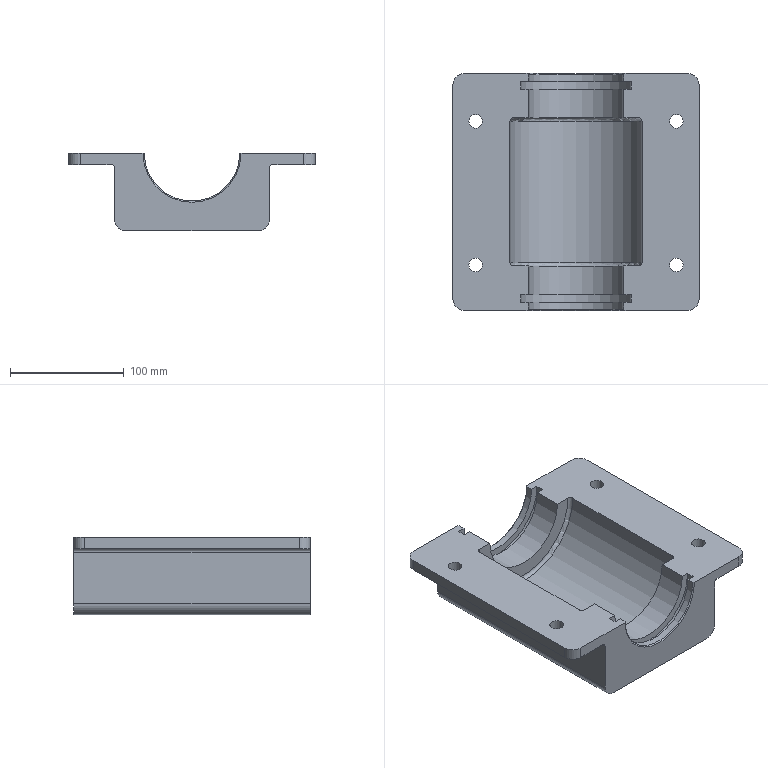Part | NX | features DATUM_CSYS 10, SKETCH 9, EXTRACT_FACE 6, HOLE PACKAGE 6, SIMPLE HOLE 6, BLEND 4, Instance Feature 4, EXTRUDE 2, Pattern Feature 2, SYMBOLIC_THREAD 2, CHAMFER 1, DATUM_PLANE 1, SWP104 1 | 1 solid | 44 faces | box 216 x 208 x 68 mm | volume 1158668 mm3 | cylinder 21 | plane 17 | cone 4 | torus 2 | commonest cylinder face diameters 20 x6 12 x4 84 x4 6 x2 8.5 x2 97 x2
STEP:
#1=CARTESIAN_POINT('',(166.,0.,68.));
#2=VERTEX_POINT('',#1);
#3=CARTESIAN_POINT('',(111.,0.,68.));
#4=VERTEX_POINT('',#3);
#5=CARTESIAN_POINT('',(176.,0.,68.));
#6=DIRECTION('',(-1.,0.,0.));
#7=VECTOR('',#6,1000.);
#8=LINE('',#5,#7);
#9=EDGE_CURVE('',#2,#4,#8,.T.);
#10=ORIENTED_EDGE('',*,*,#9,.T.);
#11=CARTESIAN_POINT('',(25.,0.,68.));
#12=VERTEX_POINT('',#11);
#13=CARTESIAN_POINT('',(68.,0.,68.));
#14=DIRECTION('',(0.,1.,0.));
#15=DIRECTION('',(-1.,0.,0.));
#16=AXIS2_PLACEMENT_3D('',#13,#14,#15);
#17=CIRCLE('',#16,43.);
#18=EDGE_CURVE('',#4,#12,#17,.T.);
#19=ORIENTED_EDGE('',*,*,#18,.T.);
#20=CARTESIAN_POINT('',(-30.,0.,68.));
#21=VERTEX_POINT('',#20);
#22=CARTESIAN_POINT('',(176.,0.,68.));
#23=DIRECTION('',(-1.,0.,0.));
#24=VECTOR('',#23,1000.);
#25=LINE('',#22,#24);
#26=EDGE_CURVE('',#12,#21,#25,.T.);
#27=ORIENTED_EDGE('',*,*,#26,.T.);
#28=CARTESIAN_POINT('',(-30.,0.,58.));
#29=VERTEX_POINT('',#28);
#30=CARTESIAN_POINT('',(-30.,0.,58.));
#31=DIRECTION('',(0.,0.,-1.));
#32=VECTOR('',#31,1000.);
#33=LINE('',#30,#32);
#34=EDGE_CURVE('',#21,#29,#33,.T.);
#35=ORIENTED_EDGE('',*,*,#34,.T.);
#36=CARTESIAN_POINT('',(-3.,0.,58.));
#37=VERTEX_POINT('',#36);
#38=CARTESIAN_POINT('',(-40.,0.,58.));
#39=DIRECTION('',(1.,0.,0.));
#40=VECTOR('',#39,1000.);
#41=LINE('',#38,#40);
#42=EDGE_CURVE('',#29,#37,#41,.T.);
#43=ORIENTED_EDGE('',*,*,#42,.T.);
#44=CARTESIAN_POINT('',(0.,0.,55.));
#45=VERTEX_POINT('',#44);
#46=CARTESIAN_POINT('',(-3.,0.,55.));
#47=DIRECTION('',(0.,1.,0.));
#48=DIRECTION('',(-1.,0.,0.));
#49=AXIS2_PLACEMENT_3D('',#46,#47,#48);
#50=CIRCLE('',#49,3.);
#51=EDGE_CURVE('',#37,#45,#50,.T.);
#52=ORIENTED_EDGE('',*,*,#51,.T.);
#53=CARTESIAN_POINT('',(0.,0.,10.));
#54=VERTEX_POINT('',#53);
#55=CARTESIAN_POINT('',(0.,0.,10.));
#56=DIRECTION('',(0.,0.,-1.));
#57=VECTOR('',#56,1000.);
#58=LINE('',#55,#57);
#59=EDGE_CURVE('',#45,#54,#58,.T.);
#60=ORIENTED_EDGE('',*,*,#59,.T.);
#61=CARTESIAN_POINT('',(10.,0.,0.));
#62=VERTEX_POINT('',#61);
#63=CARTESIAN_POINT('',(10.,0.,10.));
#64=DIRECTION('',(0.,1.,0.));
#65=DIRECTION('',(-1.,0.,0.));
#66=AXIS2_PLACEMENT_3D('',#63,#64,#65);
#67=CIRCLE('',#66,10.);
#68=EDGE_CURVE('',#54,#62,#67,.F.);
#69=ORIENTED_EDGE('',*,*,#68,.T.);
#70=CARTESIAN_POINT('',(126.,0.,0.));
#71=VERTEX_POINT('',#70);
#72=CARTESIAN_POINT('',(0.,0.,0.));
#73=DIRECTION('',(1.,0.,0.));
#74=VECTOR('',#73,1000.);
#75=LINE('',#72,#74);
#76=EDGE_CURVE('',#62,#71,#75,.T.);
#77=ORIENTED_EDGE('',*,*,#76,.T.);
#78=CARTESIAN_POINT('',(136.,0.,10.));
#79=VERTEX_POINT('',#78);
#80=CARTESIAN_POINT('',(126.,0.,10.));
#81=DIRECTION('',(0.,1.,0.));
#82=DIRECTION('',(-1.,0.,0.));
#83=AXIS2_PLACEMENT_3D('',#80,#81,#82);
#84=CIRCLE('',#83,10.);
#85=EDGE_CURVE('',#71,#79,#84,.F.);
#86=ORIENTED_EDGE('',*,*,#85,.T.);
#87=CARTESIAN_POINT('',(136.,0.,55.));
#88=VERTEX_POINT('',#87);
#89=CARTESIAN_POINT('',(136.,0.,10.));
#90=DIRECTION('',(0.,0.,-1.));
#91=VECTOR('',#90,1000.);
#92=LINE('',#89,#91);
#93=EDGE_CURVE('',#88,#79,#92,.T.);
#94=ORIENTED_EDGE('',*,*,#93,.F.);
#95=CARTESIAN_POINT('',(139.,0.,58.));
#96=VERTEX_POINT('',#95);
#97=CARTESIAN_POINT('',(139.,0.,55.));
#98=DIRECTION('',(0.,1.,0.));
#99=DIRECTION('',(-1.,0.,0.));
#100=AXIS2_PLACEMENT_3D('',#97,#98,#99);
#101=CIRCLE('',#100,3.);
#102=EDGE_CURVE('',#88,#96,#101,.T.);
#103=ORIENTED_EDGE('',*,*,#102,.T.);
#104=CARTESIAN_POINT('',(166.,0.,58.));
#105=VERTEX_POINT('',#104);
#106=CARTESIAN_POINT('',(136.,0.,58.));
#107=DIRECTION('',(1.,0.,0.));
#108=VECTOR('',#107,1000.);
#109=LINE('',#106,#108);
#110=EDGE_CURVE('',#96,#105,#109,.T.);
#111=ORIENTED_EDGE('',*,*,#110,.T.);
#112=CARTESIAN_POINT('',(166.,0.,68.));
#113=DIRECTION('',(0.,0.,1.));
#114=VECTOR('',#113,1000.);
#115=LINE('',#112,#114);
#116=EDGE_CURVE('',#105,#2,#115,.T.);
#117=ORIENTED_EDGE('',*,*,#116,.T.);
#118=EDGE_LOOP('',(#10,#19,#27,#35,#43,#52,#60,#69,#77,#86,#94,#103,#111,#117));
#119=FACE_BOUND('',#118,.T.);
#120=CARTESIAN_POINT('',(0.,0.,10.));
#121=DIRECTION('',(0.,1.,0.));
#122=DIRECTION('',(-1.,0.,0.));
#123=AXIS2_PLACEMENT_3D('',#120,#121,#122);
#124=PLANE('',#123);
#125=ADVANCED_FACE('',(#119),#124,.F.);
#126=CARTESIAN_POINT('',(-26.,166.,68.));
#127=VERTEX_POINT('',#126);
#128=CARTESIAN_POINT('',(-20.,166.,68.));
#129=DIRECTION('',(0.,0.,-1.));
#130=DIRECTION('',(-1.,0.,0.));
#131=AXIS2_PLACEMENT_3D('',#128,#129,#130);
#132=CIRCLE('',#131,6.);
#133=EDGE_CURVE('',#127,#127,#132,.T.);
#134=ORIENTED_EDGE('',*,*,#133,.T.);
#135=EDGE_LOOP('',(#134));
#136=FACE_BOUND('',#135,.T.);
#137=CARTESIAN_POINT('',(-26.,40.,68.));
#138=VERTEX_POINT('',#137);
#139=CARTESIAN_POINT('',(-20.,40.,68.));
#140=DIRECTION('',(0.,0.,-1.));
#141=DIRECTION('',(-1.,0.,0.));
#142=AXIS2_PLACEMENT_3D('',#139,#140,#141);
#143=CIRCLE('',#142,6.);
#144=EDGE_CURVE('',#138,#138,#143,.T.);
#145=ORIENTED_EDGE('',*,*,#144,.T.);
#146=EDGE_LOOP('',(#145));
#147=FACE_BOUND('',#146,.T.);
#148=ORIENTED_EDGE('',*,*,#26,.F.);
#149=CARTESIAN_POINT('',(26.,1.,68.));
#150=VERTEX_POINT('',#149);
#151=CARTESIAN_POINT('',(68.,43.,68.));
#152=DIRECTION('',(-0.7071,-0.7071,0.));
#153=VECTOR('',#152,1000.);
#154=LINE('',#151,#153);
#155=EDGE_CURVE('',#12,#150,#154,.F.);
#156=ORIENTED_EDGE('',*,*,#155,.T.);
#157=CARTESIAN_POINT('',(26.,7.,68.));
#158=VERTEX_POINT('',#157);
#159=CARTESIAN_POINT('',(26.,0.,68.));
#160=DIRECTION('',(0.,-1.,0.));
#161=VECTOR('',#160,1000.);
#162=LINE('',#159,#161);
#163=EDGE_CURVE('',#158,#150,#162,.T.);
#164=ORIENTED_EDGE('',*,*,#163,.F.);
#165=CARTESIAN_POINT('',(19.5,7.,68.));
#166=VERTEX_POINT('',#165);
#167=CARTESIAN_POINT('',(176.,7.,68.));
#168=DIRECTION('',(1.,0.,0.));
#169=VECTOR('',#168,1000.);
#170=LINE('',#167,#169);
#171=EDGE_CURVE('',#166,#158,#170,.T.);
#172=ORIENTED_EDGE('',*,*,#171,.F.);
#173=CARTESIAN_POINT('',(19.5,14.,68.));
#174=VERTEX_POINT('',#173);
#175=CARTESIAN_POINT('',(19.5,0.,68.));
#176=DIRECTION('',(0.,-1.,0.));
#177=VECTOR('',#176,1000.);
#178=LINE('',#175,#177);
#179=EDGE_CURVE('',#174,#166,#178,.T.);
#180=ORIENTED_EDGE('',*,*,#179,.F.);
#181=CARTESIAN_POINT('',(26.,14.,68.));
#182=VERTEX_POINT('',#181);
#183=CARTESIAN_POINT('',(176.,14.,68.));
#184=DIRECTION('',(-1.,0.,0.));
#185=VECTOR('',#184,1000.);
#186=LINE('',#183,#185);
#187=EDGE_CURVE('',#182,#174,#186,.T.);
#188=ORIENTED_EDGE('',*,*,#187,.F.);
#189=CARTESIAN_POINT('',(26.,39.,68.));
#190=VERTEX_POINT('',#189);
#191=CARTESIAN_POINT('',(26.,0.,68.));
#192=DIRECTION('',(0.,-1.,0.));
#193=VECTOR('',#192,1000.);
#194=LINE('',#191,#193);
#195=EDGE_CURVE('',#190,#182,#194,.T.);
#196=ORIENTED_EDGE('',*,*,#195,.F.);
#197=CARTESIAN_POINT('',(13.,39.,68.));
#198=VERTEX_POINT('',#197);
#199=CARTESIAN_POINT('',(176.,39.,68.));
#200=DIRECTION('',(1.,0.,0.));
#201=VECTOR('',#200,1000.);
#202=LINE('',#199,#201);
#203=EDGE_CURVE('',#198,#190,#202,.T.);
#204=ORIENTED_EDGE('',*,*,#203,.F.);
#205=CARTESIAN_POINT('',(10.,42.,68.));
#206=VERTEX_POINT('',#205);
#207=CARTESIAN_POINT('',(13.,42.,68.));
#208=DIRECTION('',(0.,0.,1.));
#209=DIRECTION('',(1.,0.,0.));
#210=AXIS2_PLACEMENT_3D('',#207,#208,#209);
#211=CIRCLE('',#210,3.);
#212=EDGE_CURVE('',#198,#206,#211,.F.);
#213=ORIENTED_EDGE('',*,*,#212,.T.);
#214=CARTESIAN_POINT('',(10.,166.,68.));
#215=VERTEX_POINT('',#214);
#216=CARTESIAN_POINT('',(10.,0.,68.));
#217=DIRECTION('',(0.,-1.,0.));
#218=VECTOR('',#217,1000.);
#219=LINE('',#216,#218);
#220=EDGE_CURVE('',#215,#206,#219,.T.);
#221=ORIENTED_EDGE('',*,*,#220,.F.);
#222=CARTESIAN_POINT('',(13.,169.,68.));
#223=VERTEX_POINT('',#222);
#224=CARTESIAN_POINT('',(13.,166.,68.));
#225=DIRECTION('',(0.,0.,1.));
#226=DIRECTION('',(1.,0.,0.));
#227=AXIS2_PLACEMENT_3D('',#224,#225,#226);
#228=CIRCLE('',#227,3.);
#229=EDGE_CURVE('',#215,#223,#228,.F.);
#230=ORIENTED_EDGE('',*,*,#229,.T.);
#231=CARTESIAN_POINT('',(26.,169.,68.));
#232=VERTEX_POINT('',#231);
#233=CARTESIAN_POINT('',(176.,169.,68.));
#234=DIRECTION('',(-1.,0.,0.));
#235=VECTOR('',#234,1000.);
#236=LINE('',#233,#235);
#237=EDGE_CURVE('',#232,#223,#236,.T.);
#238=ORIENTED_EDGE('',*,*,#237,.F.);
#239=CARTESIAN_POINT('',(26.,194.,68.));
#240=VERTEX_POINT('',#239);
#241=CARTESIAN_POINT('',(26.,0.,68.));
#242=DIRECTION('',(0.,-1.,0.));
#243=VECTOR('',#242,1000.);
#244=LINE('',#241,#243);
#245=EDGE_CURVE('',#240,#232,#244,.T.);
#246=ORIENTED_EDGE('',*,*,#245,.F.);
#247=CARTESIAN_POINT('',(19.5,194.,68.));
#248=VERTEX_POINT('',#247);
#249=CARTESIAN_POINT('',(176.,194.,68.));
#250=DIRECTION('',(1.,0.,0.));
#251=VECTOR('',#250,1000.);
#252=LINE('',#249,#251);
#253=EDGE_CURVE('',#248,#240,#252,.T.);
#254=ORIENTED_EDGE('',*,*,#253,.F.);
#255=CARTESIAN_POINT('',(19.5,201.,68.));
#256=VERTEX_POINT('',#255);
#257=CARTESIAN_POINT('',(19.5,0.,68.));
#258=DIRECTION('',(0.,-1.,0.));
#259=VECTOR('',#258,1000.);
#260=LINE('',#257,#259);
#261=EDGE_CURVE('',#256,#248,#260,.T.);
#262=ORIENTED_EDGE('',*,*,#261,.F.);
#263=CARTESIAN_POINT('',(26.,201.,68.));
#264=VERTEX_POINT('',#263);
#265=CARTESIAN_POINT('',(176.,201.,68.));
#266=DIRECTION('',(-1.,0.,0.));
#267=VECTOR('',#266,1000.);
#268=LINE('',#265,#267);
#269=EDGE_CURVE('',#264,#256,#268,.T.);
#270=ORIENTED_EDGE('',*,*,#269,.F.);
#271=CARTESIAN_POINT('',(26.,207.,68.));
#272=VERTEX_POINT('',#271);
#273=CARTESIAN_POINT('',(26.,0.,68.));
#274=DIRECTION('',(0.,-1.,0.));
#275=VECTOR('',#274,1000.);
#276=LINE('',#273,#275);
#277=EDGE_CURVE('',#272,#264,#276,.T.);
#278=ORIENTED_EDGE('',*,*,#277,.F.);
#279=CARTESIAN_POINT('',(25.,208.,68.));
#280=VERTEX_POINT('',#279);
#281=CARTESIAN_POINT('',(68.,165.,68.));
#282=DIRECTION('',(0.7071,-0.7071,0.));
#283=VECTOR('',#282,1000.);
#284=LINE('',#281,#283);
#285=EDGE_CURVE('',#272,#280,#284,.F.);
#286=ORIENTED_EDGE('',*,*,#285,.T.);
#287=CARTESIAN_POINT('',(-30.,208.,68.));
#288=VERTEX_POINT('',#287);
#289=CARTESIAN_POINT('',(176.,208.,68.));
#290=DIRECTION('',(-1.,0.,0.));
#291=VECTOR('',#290,1000.);
#292=LINE('',#289,#291);
#293=EDGE_CURVE('',#280,#288,#292,.T.);
#294=ORIENTED_EDGE('',*,*,#293,.T.);
#295=CARTESIAN_POINT('',(-40.,198.,68.));
#296=VERTEX_POINT('',#295);
#297=CARTESIAN_POINT('',(-30.,198.,68.));
#298=DIRECTION('',(0.,0.,1.));
#299=DIRECTION('',(1.,0.,0.));
#300=AXIS2_PLACEMENT_3D('',#297,#298,#299);
#301=CIRCLE('',#300,10.);
#302=EDGE_CURVE('',#288,#296,#301,.T.);
#303=ORIENTED_EDGE('',*,*,#302,.T.);
#304=CARTESIAN_POINT('',(-40.,10.,68.));
#305=VERTEX_POINT('',#304);
#306=CARTESIAN_POINT('',(-40.,208.,68.));
#307=DIRECTION('',(0.,-1.,0.));
#308=VECTOR('',#307,1000.);
#309=LINE('',#306,#308);
#310=EDGE_CURVE('',#296,#305,#309,.T.);
#311=ORIENTED_EDGE('',*,*,#310,.T.);
#312=CARTESIAN_POINT('',(-30.,10.,68.));
#313=DIRECTION('',(0.,0.,1.));
#314=DIRECTION('',(1.,0.,0.));
#315=AXIS2_PLACEMENT_3D('',#312,#313,#314);
#316=CIRCLE('',#315,10.);
#317=EDGE_CURVE('',#305,#21,#316,.T.);
#318=ORIENTED_EDGE('',*,*,#317,.T.);
#319=EDGE_LOOP('',(#148,#156,#164,#172,#180,#188,#196,#204,#213,#221,#230,#238,#246,#254,#262,#270,#278,#286,#294,#303,#311,#318));
#320=FACE_BOUND('',#319,.T.);
#321=CARTESIAN_POINT('',(176.,208.,68.));
#322=DIRECTION('',(0.,0.,1.));
#323=DIRECTION('',(1.,0.,0.));
#324=AXIS2_PLACEMENT_3D('',#321,#322,#323);
#325=PLANE('',#324);
#326=ADVANCED_FACE('',(#136,#147,#320),#325,.T.);
#327=ORIENTED_EDGE('',*,*,#59,.F.);
#328=CARTESIAN_POINT('',(0.,208.,55.));
#329=VERTEX_POINT('',#328);
#330=CARTESIAN_POINT('',(0.,208.,55.));
#331=DIRECTION('',(0.,-1.,0.));
#332=VECTOR('',#331,1000.);
#333=LINE('',#330,#332);
#334=EDGE_CURVE('',#45,#329,#333,.F.);
#335=ORIENTED_EDGE('',*,*,#334,.T.);
#336=CARTESIAN_POINT('',(0.,208.,10.));
#337=VERTEX_POINT('',#336);
#338=CARTESIAN_POINT('',(0.,208.,10.));
#339=DIRECTION('',(0.,0.,-1.));
#340=VECTOR('',#339,1000.);
#341=LINE('',#338,#340);
#342=EDGE_CURVE('',#329,#337,#341,.T.);
#343=ORIENTED_EDGE('',*,*,#342,.T.);
#344=CARTESIAN_POINT('',(0.,208.,10.));
#345=DIRECTION('',(0.,-1.,0.));
#346=VECTOR('',#345,1000.);
#347=LINE('',#344,#346);
#348=EDGE_CURVE('',#337,#54,#347,.T.);
#349=ORIENTED_EDGE('',*,*,#348,.T.);
#350=EDGE_LOOP('',(#327,#335,#343,#349));
#351=FACE_BOUND('',#350,.T.);
#352=CARTESIAN_POINT('',(0.,208.,10.));
#353=DIRECTION('',(1.,0.,0.));
#354=DIRECTION('',(0.,1.,0.));
#355=AXIS2_PLACEMENT_3D('',#352,#353,#354);
#356=PLANE('',#355);
#357=ADVANCED_FACE('',(#351),#356,.F.);
#358=CARTESIAN_POINT('',(136.,208.,55.));
#359=VERTEX_POINT('',#358);
#360=CARTESIAN_POINT('',(136.,208.,10.));
#361=VERTEX_POINT('',#360);
#362=CARTESIAN_POINT('',(136.,208.,10.));
#363=DIRECTION('',(0.,0.,-1.));
#364=VECTOR('',#363,1000.);
#365=LINE('',#362,#364);
#366=EDGE_CURVE('',#359,#361,#365,.T.);
#367=ORIENTED_EDGE('',*,*,#366,.F.);
#368=CARTESIAN_POINT('',(136.,0.,55.));
#369=DIRECTION('',(0.,-1.,0.));
#370=VECTOR('',#369,1000.);
#371=LINE('',#368,#370);
#372=EDGE_CURVE('',#359,#88,#371,.T.);
#373=ORIENTED_EDGE('',*,*,#372,.T.);
#374=ORIENTED_EDGE('',*,*,#93,.T.);
#375=CARTESIAN_POINT('',(136.,0.,10.));
#376=DIRECTION('',(0.,1.,0.));
#377=VECTOR('',#376,1000.);
#378=LINE('',#375,#377);
#379=EDGE_CURVE('',#79,#361,#378,.T.);
#380=ORIENTED_EDGE('',*,*,#379,.T.);
#381=EDGE_LOOP('',(#367,#373,#374,#380));
#382=FACE_BOUND('',#381,.T.);
#383=CARTESIAN_POINT('',(136.,0.,10.));
#384=DIRECTION('',(-1.,0.,0.));
#385=DIRECTION('',(0.,0.,1.));
#386=AXIS2_PLACEMENT_3D('',#383,#384,#385);
#387=PLANE('',#386);
#388=ADVANCED_FACE('',(#382),#387,.F.);
#389=ORIENTED_EDGE('',*,*,#293,.F.);
#390=CARTESIAN_POINT('',(111.,208.,68.));
#391=VERTEX_POINT('',#390);
#392=CARTESIAN_POINT('',(68.,208.,68.));
#393=DIRECTION('',(0.,-1.,0.));
#394=DIRECTION('',(1.,0.,0.));
#395=AXIS2_PLACEMENT_3D('',#392,#393,#394);
#396=CIRCLE('',#395,43.);
#397=EDGE_CURVE('',#280,#391,#396,.T.);
#398=ORIENTED_EDGE('',*,*,#397,.T.);
#399=CARTESIAN_POINT('',(166.,208.,68.));
#400=VERTEX_POINT('',#399);
#401=CARTESIAN_POINT('',(176.,208.,68.));
#402=DIRECTION('',(-1.,0.,0.));
#403=VECTOR('',#402,1000.);
#404=LINE('',#401,#403);
#405=EDGE_CURVE('',#400,#391,#404,.T.);
#406=ORIENTED_EDGE('',*,*,#405,.F.);
#407=CARTESIAN_POINT('',(166.,208.,58.));
#408=VERTEX_POINT('',#407);
#409=CARTESIAN_POINT('',(166.,208.,58.));
#410=DIRECTION('',(0.,0.,1.));
#411=VECTOR('',#410,1000.);
#412=LINE('',#409,#411);
#413=EDGE_CURVE('',#400,#408,#412,.F.);
#414=ORIENTED_EDGE('',*,*,#413,.T.);
#415=CARTESIAN_POINT('',(139.,208.,58.));
#416=VERTEX_POINT('',#415);
#417=CARTESIAN_POINT('',(136.,208.,58.));
#418=DIRECTION('',(1.,0.,0.));
#419=VECTOR('',#418,1000.);
#420=LINE('',#417,#419);
#421=EDGE_CURVE('',#416,#408,#420,.T.);
#422=ORIENTED_EDGE('',*,*,#421,.F.);
#423=CARTESIAN_POINT('',(139.,208.,55.));
#424=DIRECTION('',(0.,-1.,0.));
#425=DIRECTION('',(1.,0.,0.));
#426=AXIS2_PLACEMENT_3D('',#423,#424,#425);
#427=CIRCLE('',#426,3.);
#428=EDGE_CURVE('',#416,#359,#427,.T.);
#429=ORIENTED_EDGE('',*,*,#428,.T.);
#430=ORIENTED_EDGE('',*,*,#366,.T.);
#431=CARTESIAN_POINT('',(126.,208.,0.));
#432=VERTEX_POINT('',#431);
#433=CARTESIAN_POINT('',(126.,208.,10.));
#434=DIRECTION('',(0.,-1.,0.));
#435=DIRECTION('',(1.,0.,0.));
#436=AXIS2_PLACEMENT_3D('',#433,#434,#435);
#437=CIRCLE('',#436,10.);
#438=EDGE_CURVE('',#361,#432,#437,.F.);
#439=ORIENTED_EDGE('',*,*,#438,.T.);
#440=CARTESIAN_POINT('',(10.,208.,0.));
#441=VERTEX_POINT('',#440);
#442=CARTESIAN_POINT('',(136.,208.,0.));
#443=DIRECTION('',(-1.,0.,0.));
#444=VECTOR('',#443,1000.);
#445=LINE('',#442,#444);
#446=EDGE_CURVE('',#432,#441,#445,.T.);
#447=ORIENTED_EDGE('',*,*,#446,.T.);
#448=CARTESIAN_POINT('',(10.,208.,10.));
#449=DIRECTION('',(0.,-1.,0.));
#450=DIRECTION('',(1.,0.,0.));
#451=AXIS2_PLACEMENT_3D('',#448,#449,#450);
#452=CIRCLE('',#451,10.);
#453=EDGE_CURVE('',#441,#337,#452,.F.);
#454=ORIENTED_EDGE('',*,*,#453,.T.);
#455=ORIENTED_EDGE('',*,*,#342,.F.);
#456=CARTESIAN_POINT('',(-3.,208.,58.));
#457=VERTEX_POINT('',#456);
#458=CARTESIAN_POINT('',(-3.,208.,55.));
#459=DIRECTION('',(0.,-1.,0.));
#460=DIRECTION('',(1.,0.,0.));
#461=AXIS2_PLACEMENT_3D('',#458,#459,#460);
#462=CIRCLE('',#461,3.);
#463=EDGE_CURVE('',#329,#457,#462,.T.);
#464=ORIENTED_EDGE('',*,*,#463,.T.);
#465=CARTESIAN_POINT('',(-30.,208.,58.));
#466=VERTEX_POINT('',#465);
#467=CARTESIAN_POINT('',(-40.,208.,58.));
#468=DIRECTION('',(1.,0.,0.));
#469=VECTOR('',#468,1000.);
#470=LINE('',#467,#469);
#471=EDGE_CURVE('',#466,#457,#470,.T.);
#472=ORIENTED_EDGE('',*,*,#471,.F.);
#473=CARTESIAN_POINT('',(-30.,208.,68.));
#474=DIRECTION('',(0.,0.,-1.));
#475=VECTOR('',#474,1000.);
#476=LINE('',#473,#475);
#477=EDGE_CURVE('',#466,#288,#476,.F.);
#478=ORIENTED_EDGE('',*,*,#477,.T.);
#479=EDGE_LOOP('',(#389,#398,#406,#414,#422,#429,#430,#439,#447,#454,#455,#464,#472,#478));
#480=FACE_BOUND('',#479,.T.);
#481=CARTESIAN_POINT('',(136.,208.,10.));
#482=DIRECTION('',(0.,-1.,0.));
#483=DIRECTION('',(1.,0.,0.));
#484=AXIS2_PLACEMENT_3D('',#481,#482,#483);
#485=PLANE('',#484);
#486=ADVANCED_FACE('',(#480),#485,.F.);
#487=CARTESIAN_POINT('',(108.25,182.,0.));
#488=VERTEX_POINT('',#487);
#489=CARTESIAN_POINT('',(104.,182.,0.));
#490=DIRECTION('',(0.,0.,1.));
#491=DIRECTION('',(1.,0.,0.));
#492=AXIS2_PLACEMENT_3D('',#489,#490,#491);
#493=CIRCLE('',#492,4.25);
#494=EDGE_CURVE('',#488,#488,#493,.T.);
#495=ORIENTED_EDGE('',*,*,#494,.T.);
#496=EDGE_LOOP('',(#495));
#497=FACE_BOUND('',#496,.T.);
#498=CARTESIAN_POINT('',(36.25,182.,0.));
#499=VERTEX_POINT('',#498);
#500=CARTESIAN_POINT('',(32.,182.,0.));
#501=DIRECTION('',(0.,0.,1.));
#502=DIRECTION('',(1.,0.,0.));
#503=AXIS2_PLACEMENT_3D('',#500,#501,#502);
#504=CIRCLE('',#503,4.25);
#505=EDGE_CURVE('',#499,#499,#504,.T.);
#506=ORIENTED_EDGE('',*,*,#505,.T.);
#507=EDGE_LOOP('',(#506));
#508=FACE_BOUND('',#507,.T.);
#509=ORIENTED_EDGE('',*,*,#446,.F.);
#510=CARTESIAN_POINT('',(126.,0.,0.));
#511=DIRECTION('',(0.,1.,0.));
#512=VECTOR('',#511,1000.);
#513=LINE('',#510,#512);
#514=EDGE_CURVE('',#432,#71,#513,.F.);
#515=ORIENTED_EDGE('',*,*,#514,.T.);
#516=ORIENTED_EDGE('',*,*,#76,.F.);
#517=CARTESIAN_POINT('',(10.,0.,0.));
#518=DIRECTION('',(0.,-1.,0.));
#519=VECTOR('',#518,1000.);
#520=LINE('',#517,#519);
#521=EDGE_CURVE('',#62,#441,#520,.F.);
#522=ORIENTED_EDGE('',*,*,#521,.T.);
#523=EDGE_LOOP('',(#509,#515,#516,#522));
#524=FACE_BOUND('',#523,.T.);
#525=CARTESIAN_POINT('',(0.,0.,0.));
#526=DIRECTION('',(0.,0.,1.));
#527=DIRECTION('',(1.,0.,0.));
#528=AXIS2_PLACEMENT_3D('',#525,#526,#527);
#529=PLANE('',#528);
#530=ADVANCED_FACE('',(#497,#508,#524),#529,.F.);
#531=CARTESIAN_POINT('',(-40.,198.,58.));
#532=VERTEX_POINT('',#531);
#533=CARTESIAN_POINT('',(-40.,10.,58.));
#534=VERTEX_POINT('',#533);
#535=CARTESIAN_POINT('',(-40.,208.,58.));
#536=DIRECTION('',(0.,-1.,0.));
#537=VECTOR('',#536,1000.);
#538=LINE('',#535,#537);
#539=EDGE_CURVE('',#532,#534,#538,.T.);
#540=ORIENTED_EDGE('',*,*,#539,.T.);
#541=CARTESIAN_POINT('',(-40.,10.,68.));
#542=DIRECTION('',(0.,0.,-1.));
#543=VECTOR('',#542,1000.);
#544=LINE('',#541,#543);
#545=EDGE_CURVE('',#534,#305,#544,.F.);
#546=ORIENTED_EDGE('',*,*,#545,.T.);
#547=ORIENTED_EDGE('',*,*,#310,.F.);
#548=CARTESIAN_POINT('',(-40.,198.,58.));
#549=DIRECTION('',(0.,0.,-1.));
#550=VECTOR('',#549,1000.);
#551=LINE('',#548,#550);
#552=EDGE_CURVE('',#296,#532,#551,.T.);
#553=ORIENTED_EDGE('',*,*,#552,.T.);
#554=EDGE_LOOP('',(#540,#546,#547,#553));
#555=FACE_BOUND('',#554,.T.);
#556=CARTESIAN_POINT('',(-40.,208.,68.));
#557=DIRECTION('',(-1.,0.,0.));
#558=DIRECTION('',(0.,0.,1.));
#559=AXIS2_PLACEMENT_3D('',#556,#557,#558);
#560=PLANE('',#559);
#561=ADVANCED_FACE('',(#555),#560,.T.);
#562=CARTESIAN_POINT('',(-26.,166.,58.));
#563=VERTEX_POINT('',#562);
#564=CARTESIAN_POINT('',(-20.,166.,58.));
#565=DIRECTION('',(0.,0.,-1.));
#566=DIRECTION('',(-1.,0.,0.));
#567=AXIS2_PLACEMENT_3D('',#564,#565,#566);
#568=CIRCLE('',#567,6.);
#569=EDGE_CURVE('',#563,#563,#568,.T.);
#570=ORIENTED_EDGE('',*,*,#569,.F.);
#571=EDGE_LOOP('',(#570));
#572=FACE_BOUND('',#571,.T.);
#573=CARTESIAN_POINT('',(-26.,40.,58.));
#574=VERTEX_POINT('',#573);
#575=CARTESIAN_POINT('',(-20.,40.,58.));
#576=DIRECTION('',(0.,0.,-1.));
#577=DIRECTION('',(-1.,0.,0.));
#578=AXIS2_PLACEMENT_3D('',#575,#576,#577);
#579=CIRCLE('',#578,6.);
#580=EDGE_CURVE('',#574,#574,#579,.T.);
#581=ORIENTED_EDGE('',*,*,#580,.F.);
#582=EDGE_LOOP('',(#581));
#583=FACE_BOUND('',#582,.T.);
#584=ORIENTED_EDGE('',*,*,#42,.F.);
#585=CARTESIAN_POINT('',(-30.,10.,58.));
#586=DIRECTION('',(0.,0.,-1.));
#587=DIRECTION('',(-1.,0.,0.));
#588=AXIS2_PLACEMENT_3D('',#585,#586,#587);
#589=CIRCLE('',#588,10.);
#590=EDGE_CURVE('',#29,#534,#589,.T.);
#591=ORIENTED_EDGE('',*,*,#590,.T.);
#592=ORIENTED_EDGE('',*,*,#539,.F.);
#593=CARTESIAN_POINT('',(-30.,198.,58.));
#594=DIRECTION('',(0.,0.,-1.));
#595=DIRECTION('',(-1.,0.,0.));
#596=AXIS2_PLACEMENT_3D('',#593,#594,#595);
#597=CIRCLE('',#596,10.);
#598=EDGE_CURVE('',#532,#466,#597,.T.);
#599=ORIENTED_EDGE('',*,*,#598,.T.);
#600=ORIENTED_EDGE('',*,*,#471,.T.);
#601=CARTESIAN_POINT('',(-3.,208.,58.));
#602=DIRECTION('',(0.,-1.,0.));
#603=VECTOR('',#602,1000.);
#604=LINE('',#601,#603);
#605=EDGE_CURVE('',#457,#37,#604,.T.);
#606=ORIENTED_EDGE('',*,*,#605,.T.);
#607=EDGE_LOOP('',(#584,#591,#592,#599,#600,#606));
#608=FACE_BOUND('',#607,.T.);
#609=CARTESIAN_POINT('',(-40.,208.,58.));
#610=DIRECTION('',(0.,0.,-1.));
#611=DIRECTION('',(-1.,0.,0.));
#612=AXIS2_PLACEMENT_3D('',#609,#610,#611);
#613=PLANE('',#612);
#614=ADVANCED_FACE('',(#572,#583,#608),#613,.T.);
#615=CARTESIAN_POINT('',(150.,166.,58.));
#616=VERTEX_POINT('',#615);
#617=CARTESIAN_POINT('',(156.,166.,58.));
#618=DIRECTION('',(0.,0.,-1.));
#619=DIRECTION('',(-1.,0.,0.));
#620=AXIS2_PLACEMENT_3D('',#617,#618,#619);
#621=CIRCLE('',#620,6.);
#622=EDGE_CURVE('',#616,#616,#621,.T.);
#623=ORIENTED_EDGE('',*,*,#622,.F.);
#624=EDGE_LOOP('',(#623));
#625=FACE_BOUND('',#624,.T.);
#626=CARTESIAN_POINT('',(150.,40.,58.));
#627=VERTEX_POINT('',#626);
#628=CARTESIAN_POINT('',(156.,40.,58.));
#629=DIRECTION('',(0.,0.,-1.));
#630=DIRECTION('',(-1.,0.,0.));
#631=AXIS2_PLACEMENT_3D('',#628,#629,#630);
#632=CIRCLE('',#631,6.);
#633=EDGE_CURVE('',#627,#627,#632,.T.);
#634=ORIENTED_EDGE('',*,*,#633,.F.);
#635=EDGE_LOOP('',(#634));
#636=FACE_BOUND('',#635,.T.);
#637=CARTESIAN_POINT('',(176.,198.,58.));
#638=VERTEX_POINT('',#637);
#639=CARTESIAN_POINT('',(176.,10.,58.));
#640=VERTEX_POINT('',#639);
#641=CARTESIAN_POINT('',(176.,208.,58.));
#642=DIRECTION('',(0.,-1.,0.));
#643=VECTOR('',#642,1000.);
#644=LINE('',#641,#643);
#645=EDGE_CURVE('',#638,#640,#644,.T.);
#646=ORIENTED_EDGE('',*,*,#645,.T.);
#647=CARTESIAN_POINT('',(166.,10.,58.));
#648=DIRECTION('',(0.,0.,-1.));
#649=DIRECTION('',(-1.,0.,0.));
#650=AXIS2_PLACEMENT_3D('',#647,#648,#649);
#651=CIRCLE('',#650,10.);
#652=EDGE_CURVE('',#640,#105,#651,.T.);
#653=ORIENTED_EDGE('',*,*,#652,.T.);
#654=ORIENTED_EDGE('',*,*,#110,.F.);
#655=CARTESIAN_POINT('',(139.,208.,58.));
#656=DIRECTION('',(0.,-1.,0.));
#657=VECTOR('',#656,1000.);
#658=LINE('',#655,#657);
#659=EDGE_CURVE('',#96,#416,#658,.F.);
#660=ORIENTED_EDGE('',*,*,#659,.T.);
#661=ORIENTED_EDGE('',*,*,#421,.T.);
#662=CARTESIAN_POINT('',(166.,198.,58.));
#663=DIRECTION('',(0.,0.,-1.));
#664=DIRECTION('',(-1.,0.,0.));
#665=AXIS2_PLACEMENT_3D('',#662,#663,#664);
#666=CIRCLE('',#665,10.);
#667=EDGE_CURVE('',#408,#638,#666,.T.);
#668=ORIENTED_EDGE('',*,*,#667,.T.);
#669=EDGE_LOOP('',(#646,#653,#654,#660,#661,#668));
#670=FACE_BOUND('',#669,.T.);
#671=CARTESIAN_POINT('',(136.,208.,58.));
#672=DIRECTION('',(0.,0.,-1.));
#673=DIRECTION('',(-1.,0.,0.));
#674=AXIS2_PLACEMENT_3D('',#671,#672,#673);
#675=PLANE('',#674);
#676=ADVANCED_FACE('',(#625,#636,#670),#675,.T.);
#677=CARTESIAN_POINT('',(176.,198.,68.));
#678=VERTEX_POINT('',#677);
#679=CARTESIAN_POINT('',(176.,10.,68.));
#680=VERTEX_POINT('',#679);
#681=CARTESIAN_POINT('',(176.,208.,68.));
#682=DIRECTION('',(0.,-1.,0.));
#683=VECTOR('',#682,1000.);
#684=LINE('',#681,#683);
#685=EDGE_CURVE('',#678,#680,#684,.T.);
#686=ORIENTED_EDGE('',*,*,#685,.T.);
#687=CARTESIAN_POINT('',(176.,10.,58.));
#688=DIRECTION('',(0.,0.,1.));
#689=VECTOR('',#688,1000.);
#690=LINE('',#687,#689);
#691=EDGE_CURVE('',#680,#640,#690,.F.);
#692=ORIENTED_EDGE('',*,*,#691,.T.);
#693=ORIENTED_EDGE('',*,*,#645,.F.);
#694=CARTESIAN_POINT('',(176.,198.,68.));
#695=DIRECTION('',(0.,0.,1.));
#696=VECTOR('',#695,1000.);
#697=LINE('',#694,#696);
#698=EDGE_CURVE('',#638,#678,#697,.T.);
#699=ORIENTED_EDGE('',*,*,#698,.T.);
#700=EDGE_LOOP('',(#686,#692,#693,#699));
#701=FACE_BOUND('',#700,.T.);
#702=CARTESIAN_POINT('',(176.,208.,58.));
#703=DIRECTION('',(1.,0.,0.));
#704=DIRECTION('',(0.,0.,-1.));
#705=AXIS2_PLACEMENT_3D('',#702,#703,#704);
#706=PLANE('',#705);
#707=ADVANCED_FACE('',(#701),#706,.T.);
#708=CARTESIAN_POINT('',(150.,166.,68.));
#709=VERTEX_POINT('',#708);
#710=CARTESIAN_POINT('',(156.,166.,68.));
#711=DIRECTION('',(0.,0.,-1.));
#712=DIRECTION('',(-1.,0.,0.));
#713=AXIS2_PLACEMENT_3D('',#710,#711,#712);
#714=CIRCLE('',#713,6.);
#715=EDGE_CURVE('',#709,#709,#714,.T.);
#716=ORIENTED_EDGE('',*,*,#715,.T.);
#717=EDGE_LOOP('',(#716));
#718=FACE_BOUND('',#717,.T.);
#719=CARTESIAN_POINT('',(150.,40.,68.));
#720=VERTEX_POINT('',#719);
#721=CARTESIAN_POINT('',(156.,40.,68.));
#722=DIRECTION('',(0.,0.,-1.));
#723=DIRECTION('',(-1.,0.,0.));
#724=AXIS2_PLACEMENT_3D('',#721,#722,#723);
#725=CIRCLE('',#724,6.);
#726=EDGE_CURVE('',#720,#720,#725,.T.);
#727=ORIENTED_EDGE('',*,*,#726,.T.);
#728=EDGE_LOOP('',(#727));
#729=FACE_BOUND('',#728,.T.);
#730=CARTESIAN_POINT('',(110.,1.,68.));
#731=VERTEX_POINT('',#730);
#732=CARTESIAN_POINT('',(110.,7.,68.));
#733=VERTEX_POINT('',#732);
#734=CARTESIAN_POINT('',(110.,0.,68.));
#735=DIRECTION('',(0.,-1.,0.));
#736=VECTOR('',#735,1000.);
#737=LINE('',#734,#736);
#738=EDGE_CURVE('',#731,#733,#737,.F.);
#739=ORIENTED_EDGE('',*,*,#738,.F.);
#740=CARTESIAN_POINT('',(68.,43.,68.));
#741=DIRECTION('',(-0.7071,0.7071,0.));
#742=VECTOR('',#741,1000.);
#743=LINE('',#740,#742);
#744=EDGE_CURVE('',#731,#4,#743,.F.);
#745=ORIENTED_EDGE('',*,*,#744,.T.);
#746=ORIENTED_EDGE('',*,*,#9,.F.);
#747=CARTESIAN_POINT('',(166.,10.,68.));
#748=DIRECTION('',(0.,0.,1.));
#749=DIRECTION('',(1.,0.,0.));
#750=AXIS2_PLACEMENT_3D('',#747,#748,#749);
#751=CIRCLE('',#750,10.);
#752=EDGE_CURVE('',#2,#680,#751,.T.);
#753=ORIENTED_EDGE('',*,*,#752,.T.);
#754=ORIENTED_EDGE('',*,*,#685,.F.);
#755=CARTESIAN_POINT('',(166.,198.,68.));
#756=DIRECTION('',(0.,0.,1.));
#757=DIRECTION('',(1.,0.,0.));
#758=AXIS2_PLACEMENT_3D('',#755,#756,#757);
#759=CIRCLE('',#758,10.);
#760=EDGE_CURVE('',#678,#400,#759,.T.);
#761=ORIENTED_EDGE('',*,*,#760,.T.);
#762=ORIENTED_EDGE('',*,*,#405,.T.);
#763=CARTESIAN_POINT('',(110.,207.,68.));
#764=VERTEX_POINT('',#763);
#765=CARTESIAN_POINT('',(68.,165.,68.));
#766=DIRECTION('',(0.7071,0.7071,0.));
#767=VECTOR('',#766,1000.);
#768=LINE('',#765,#767);
#769=EDGE_CURVE('',#391,#764,#768,.F.);
#770=ORIENTED_EDGE('',*,*,#769,.T.);
#771=CARTESIAN_POINT('',(110.,201.,68.));
#772=VERTEX_POINT('',#771);
#773=CARTESIAN_POINT('',(110.,0.,68.));
#774=DIRECTION('',(0.,-1.,0.));
#775=VECTOR('',#774,1000.);
#776=LINE('',#773,#775);
#777=EDGE_CURVE('',#772,#764,#776,.F.);
#778=ORIENTED_EDGE('',*,*,#777,.F.);
#779=CARTESIAN_POINT('',(116.5,201.,68.));
#780=VERTEX_POINT('',#779);
#781=CARTESIAN_POINT('',(176.,201.,68.));
#782=DIRECTION('',(-1.,0.,0.));
#783=VECTOR('',#782,1000.);
#784=LINE('',#781,#783);
#785=EDGE_CURVE('',#780,#772,#784,.T.);
#786=ORIENTED_EDGE('',*,*,#785,.F.);
#787=CARTESIAN_POINT('',(116.5,194.,68.));
#788=VERTEX_POINT('',#787);
#789=CARTESIAN_POINT('',(116.5,0.,68.));
#790=DIRECTION('',(0.,-1.,0.));
#791=VECTOR('',#790,1000.);
#792=LINE('',#789,#791);
#793=EDGE_CURVE('',#788,#780,#792,.F.);
#794=ORIENTED_EDGE('',*,*,#793,.F.);
#795=CARTESIAN_POINT('',(110.,194.,68.));
#796=VERTEX_POINT('',#795);
#797=CARTESIAN_POINT('',(176.,194.,68.));
#798=DIRECTION('',(1.,0.,0.));
#799=VECTOR('',#798,1000.);
#800=LINE('',#797,#799);
#801=EDGE_CURVE('',#796,#788,#800,.T.);
#802=ORIENTED_EDGE('',*,*,#801,.F.);
#803=CARTESIAN_POINT('',(110.,169.,68.));
#804=VERTEX_POINT('',#803);
#805=CARTESIAN_POINT('',(110.,0.,68.));
#806=DIRECTION('',(0.,-1.,0.));
#807=VECTOR('',#806,1000.);
#808=LINE('',#805,#807);
#809=EDGE_CURVE('',#804,#796,#808,.F.);
#810=ORIENTED_EDGE('',*,*,#809,.F.);
#811=CARTESIAN_POINT('',(123.,169.,68.));
#812=VERTEX_POINT('',#811);
#813=CARTESIAN_POINT('',(176.,169.,68.));
#814=DIRECTION('',(-1.,0.,0.));
#815=VECTOR('',#814,1000.);
#816=LINE('',#813,#815);
#817=EDGE_CURVE('',#812,#804,#816,.T.);
#818=ORIENTED_EDGE('',*,*,#817,.F.);
#819=CARTESIAN_POINT('',(126.,166.,68.));
#820=VERTEX_POINT('',#819);
#821=CARTESIAN_POINT('',(123.,166.,68.));
#822=DIRECTION('',(0.,0.,1.));
#823=DIRECTION('',(1.,0.,0.));
#824=AXIS2_PLACEMENT_3D('',#821,#822,#823);
#825=CIRCLE('',#824,3.);
#826=EDGE_CURVE('',#812,#820,#825,.F.);
#827=ORIENTED_EDGE('',*,*,#826,.T.);
#828=CARTESIAN_POINT('',(126.,42.,68.));
#829=VERTEX_POINT('',#828);
#830=CARTESIAN_POINT('',(126.,0.,68.));
#831=DIRECTION('',(0.,-1.,0.));
#832=VECTOR('',#831,1000.);
#833=LINE('',#830,#832);
#834=EDGE_CURVE('',#829,#820,#833,.F.);
#835=ORIENTED_EDGE('',*,*,#834,.F.);
#836=CARTESIAN_POINT('',(123.,39.,68.));
#837=VERTEX_POINT('',#836);
#838=CARTESIAN_POINT('',(123.,42.,68.));
#839=DIRECTION('',(0.,0.,1.));
#840=DIRECTION('',(1.,0.,0.));
#841=AXIS2_PLACEMENT_3D('',#838,#839,#840);
#842=CIRCLE('',#841,3.);
#843=EDGE_CURVE('',#829,#837,#842,.F.);
#844=ORIENTED_EDGE('',*,*,#843,.T.);
#845=CARTESIAN_POINT('',(110.,39.,68.));
#846=VERTEX_POINT('',#845);
#847=CARTESIAN_POINT('',(176.,39.,68.));
#848=DIRECTION('',(1.,0.,0.));
#849=VECTOR('',#848,1000.);
#850=LINE('',#847,#849);
#851=EDGE_CURVE('',#846,#837,#850,.T.);
#852=ORIENTED_EDGE('',*,*,#851,.F.);
#853=CARTESIAN_POINT('',(110.,14.,68.));
#854=VERTEX_POINT('',#853);
#855=CARTESIAN_POINT('',(110.,0.,68.));
#856=DIRECTION('',(0.,-1.,0.));
#857=VECTOR('',#856,1000.);
#858=LINE('',#855,#857);
#859=EDGE_CURVE('',#854,#846,#858,.F.);
#860=ORIENTED_EDGE('',*,*,#859,.F.);
#861=CARTESIAN_POINT('',(116.5,14.,68.));
#862=VERTEX_POINT('',#861);
#863=CARTESIAN_POINT('',(176.,14.,68.));
#864=DIRECTION('',(-1.,0.,0.));
#865=VECTOR('',#864,1000.);
#866=LINE('',#863,#865);
#867=EDGE_CURVE('',#862,#854,#866,.T.);
#868=ORIENTED_EDGE('',*,*,#867,.F.);
#869=CARTESIAN_POINT('',(116.5,7.,68.));
#870=VERTEX_POINT('',#869);
#871=CARTESIAN_POINT('',(116.5,0.,68.));
#872=DIRECTION('',(0.,-1.,0.));
#873=VECTOR('',#872,1000.);
#874=LINE('',#871,#873);
#875=EDGE_CURVE('',#870,#862,#874,.F.);
#876=ORIENTED_EDGE('',*,*,#875,.F.);
#877=CARTESIAN_POINT('',(176.,7.,68.));
#878=DIRECTION('',(1.,0.,0.));
#879=VECTOR('',#878,1000.);
#880=LINE('',#877,#879);
#881=EDGE_CURVE('',#733,#870,#880,.T.);
#882=ORIENTED_EDGE('',*,*,#881,.F.);
#883=EDGE_LOOP('',(#739,#745,#746,#753,#754,#761,#762,#770,#778,#786,#794,#802,#810,#818,#827,#835,#844,#852,#860,#868,#876,#882));
#884=FACE_BOUND('',#883,.T.);
#885=CARTESIAN_POINT('',(176.,208.,68.));
#886=DIRECTION('',(0.,0.,1.));
#887=DIRECTION('',(1.,0.,0.));
#888=AXIS2_PLACEMENT_3D('',#885,#886,#887);
#889=PLANE('',#888);
#890=ADVANCED_FACE('',(#718,#729,#884),#889,.T.);
#891=ORIENTED_EDGE('',*,*,#163,.T.);
#892=CARTESIAN_POINT('',(68.,1.,68.));
#893=DIRECTION('',(0.,1.,0.));
#894=DIRECTION('',(0.,0.,1.));
#895=AXIS2_PLACEMENT_3D('',#892,#893,#894);
#896=CIRCLE('',#895,42.);
#897=EDGE_CURVE('',#150,#731,#896,.F.);
#898=ORIENTED_EDGE('',*,*,#897,.T.);
#899=ORIENTED_EDGE('',*,*,#738,.T.);
#900=CARTESIAN_POINT('',(68.,7.,68.));
#901=DIRECTION('',(0.,-1.,0.));
#902=DIRECTION('',(0.,0.,-1.));
#903=AXIS2_PLACEMENT_3D('',#900,#901,#902);
#904=CIRCLE('',#903,42.);
#905=EDGE_CURVE('',#733,#158,#904,.F.);
#906=ORIENTED_EDGE('',*,*,#905,.T.);
#907=EDGE_LOOP('',(#891,#898,#899,#906));
#908=FACE_BOUND('',#907,.T.);
#909=CARTESIAN_POINT('',(68.,0.,68.));
#910=DIRECTION('',(0.,-1.,0.));
#911=DIRECTION('',(0.,0.,-1.));
#912=AXIS2_PLACEMENT_3D('',#909,#910,#911);
#913=CYLINDRICAL_SURFACE('',#912,42.);
#914=ADVANCED_FACE('',(#908),#913,.F.);
#915=ORIENTED_EDGE('',*,*,#171,.T.);
#916=ORIENTED_EDGE('',*,*,#905,.F.);
#917=ORIENTED_EDGE('',*,*,#881,.T.);
#918=CARTESIAN_POINT('',(68.,7.,68.));
#919=DIRECTION('',(0.,-1.,0.));
#920=DIRECTION('',(0.,0.,-1.));
#921=AXIS2_PLACEMENT_3D('',#918,#919,#920);
#922=CIRCLE('',#921,48.5);
#923=EDGE_CURVE('',#870,#166,#922,.F.);
#924=ORIENTED_EDGE('',*,*,#923,.T.);
#925=EDGE_LOOP('',(#915,#916,#917,#924));
#926=FACE_BOUND('',#925,.T.);
#927=CARTESIAN_POINT('',(68.,7.,26.));
#928=DIRECTION('',(0.,-1.,0.));
#929=DIRECTION('',(0.,0.,-1.));
#930=AXIS2_PLACEMENT_3D('',#927,#928,#929);
#931=PLANE('',#930);
#932=ADVANCED_FACE('',(#926),#931,.F.);
#933=ORIENTED_EDGE('',*,*,#179,.T.);
#934=ORIENTED_EDGE('',*,*,#923,.F.);
#935=ORIENTED_EDGE('',*,*,#875,.T.);
#936=CARTESIAN_POINT('',(68.,14.,68.));
#937=DIRECTION('',(0.,-1.,0.));
#938=DIRECTION('',(0.,0.,-1.));
#939=AXIS2_PLACEMENT_3D('',#936,#937,#938);
#940=CIRCLE('',#939,48.5);
#941=EDGE_CURVE('',#862,#174,#940,.F.);
#942=ORIENTED_EDGE('',*,*,#941,.T.);
#943=EDGE_LOOP('',(#933,#934,#935,#942));
#944=FACE_BOUND('',#943,.T.);
#945=CARTESIAN_POINT('',(68.,0.,68.));
#946=DIRECTION('',(0.,-1.,0.));
#947=DIRECTION('',(0.,0.,-1.));
#948=AXIS2_PLACEMENT_3D('',#945,#946,#947);
#949=CYLINDRICAL_SURFACE('',#948,48.5);
#950=ADVANCED_FACE('',(#944),#949,.F.);
#951=ORIENTED_EDGE('',*,*,#867,.T.);
#952=CARTESIAN_POINT('',(68.,14.,68.));
#953=DIRECTION('',(0.,-1.,0.));
#954=DIRECTION('',(0.,0.,-1.));
#955=AXIS2_PLACEMENT_3D('',#952,#953,#954);
#956=CIRCLE('',#955,42.);
#957=EDGE_CURVE('',#854,#182,#956,.F.);
#958=ORIENTED_EDGE('',*,*,#957,.T.);
#959=ORIENTED_EDGE('',*,*,#187,.T.);
#960=ORIENTED_EDGE('',*,*,#941,.F.);
#961=EDGE_LOOP('',(#951,#958,#959,#960));
#962=FACE_BOUND('',#961,.T.);
#963=CARTESIAN_POINT('',(68.,14.,19.5));
#964=DIRECTION('',(0.,1.,0.));
#965=DIRECTION('',(0.,0.,1.));
#966=AXIS2_PLACEMENT_3D('',#963,#964,#965);
#967=PLANE('',#966);
#968=ADVANCED_FACE('',(#962),#967,.F.);
#969=ORIENTED_EDGE('',*,*,#195,.T.);
#970=ORIENTED_EDGE('',*,*,#957,.F.);
#971=ORIENTED_EDGE('',*,*,#859,.T.);
#972=CARTESIAN_POINT('',(68.,39.,68.));
#973=DIRECTION('',(0.,-1.,0.));
#974=DIRECTION('',(0.,0.,-1.));
#975=AXIS2_PLACEMENT_3D('',#972,#973,#974);
#976=CIRCLE('',#975,42.);
#977=EDGE_CURVE('',#846,#190,#976,.F.);
#978=ORIENTED_EDGE('',*,*,#977,.T.);
#979=EDGE_LOOP('',(#969,#970,#971,#978));
#980=FACE_BOUND('',#979,.T.);
#981=CARTESIAN_POINT('',(68.,0.,68.));
#982=DIRECTION('',(0.,-1.,0.));
#983=DIRECTION('',(0.,0.,-1.));
#984=AXIS2_PLACEMENT_3D('',#981,#982,#983);
#985=CYLINDRICAL_SURFACE('',#984,42.);
#986=ADVANCED_FACE('',(#980),#985,.F.);
#987=ORIENTED_EDGE('',*,*,#851,.T.);
#988=CARTESIAN_POINT('',(68.,39.,68.));
#989=DIRECTION('',(0.,-1.,0.));
#990=DIRECTION('',(0.,0.,-1.));
#991=AXIS2_PLACEMENT_3D('',#988,#989,#990);
#992=CIRCLE('',#991,55.);
#993=EDGE_CURVE('',#837,#198,#992,.F.);
#994=ORIENTED_EDGE('',*,*,#993,.T.);
#995=ORIENTED_EDGE('',*,*,#203,.T.);
#996=ORIENTED_EDGE('',*,*,#977,.F.);
#997=EDGE_LOOP('',(#987,#994,#995,#996));
#998=FACE_BOUND('',#997,.T.);
#999=CARTESIAN_POINT('',(68.,39.,26.));
#1000=DIRECTION('',(0.,-1.,0.));
#1001=DIRECTION('',(0.,0.,-1.));
#1002=AXIS2_PLACEMENT_3D('',#999,#1000,#1001);
#1003=PLANE('',#1002);
#1004=ADVANCED_FACE('',(#998),#1003,.F.);
#1005=ORIENTED_EDGE('',*,*,#220,.T.);
#1006=CARTESIAN_POINT('',(68.,42.,68.));
#1007=DIRECTION('',(0.,-1.,0.));
#1008=DIRECTION('',(0.,0.,-1.));
#1009=AXIS2_PLACEMENT_3D('',#1006,#1007,#1008);
#1010=CIRCLE('',#1009,58.);
#1011=EDGE_CURVE('',#206,#829,#1010,.T.);
#1012=ORIENTED_EDGE('',*,*,#1011,.T.);
#1013=ORIENTED_EDGE('',*,*,#834,.T.);
#1014=CARTESIAN_POINT('',(68.,166.,68.));
#1015=DIRECTION('',(0.,1.,0.));
#1016=DIRECTION('',(0.,0.,1.));
#1017=AXIS2_PLACEMENT_3D('',#1014,#1015,#1016);
#1018=CIRCLE('',#1017,58.);
#1019=EDGE_CURVE('',#820,#215,#1018,.T.);
#1020=ORIENTED_EDGE('',*,*,#1019,.T.);
#1021=EDGE_LOOP('',(#1005,#1012,#1013,#1020));
#1022=FACE_BOUND('',#1021,.T.);
#1023=CARTESIAN_POINT('',(68.,0.,68.));
#1024=DIRECTION('',(0.,-1.,0.));
#1025=DIRECTION('',(0.,0.,-1.));
#1026=AXIS2_PLACEMENT_3D('',#1023,#1024,#1025);
#1027=CYLINDRICAL_SURFACE('',#1026,58.);
#1028=ADVANCED_FACE('',(#1022),#1027,.F.);
#1029=ORIENTED_EDGE('',*,*,#237,.T.);
#1030=CARTESIAN_POINT('',(68.,169.,68.));
#1031=DIRECTION('',(0.,1.,0.));
#1032=DIRECTION('',(0.,0.,1.));
#1033=AXIS2_PLACEMENT_3D('',#1030,#1031,#1032);
#1034=CIRCLE('',#1033,55.);
#1035=EDGE_CURVE('',#223,#812,#1034,.F.);
#1036=ORIENTED_EDGE('',*,*,#1035,.T.);
#1037=ORIENTED_EDGE('',*,*,#817,.T.);
#1038=CARTESIAN_POINT('',(68.,169.,68.));
#1039=DIRECTION('',(0.,-1.,0.));
#1040=DIRECTION('',(0.,0.,-1.));
#1041=AXIS2_PLACEMENT_3D('',#1038,#1039,#1040);
#1042=CIRCLE('',#1041,42.);
#1043=EDGE_CURVE('',#804,#232,#1042,.F.);
#1044=ORIENTED_EDGE('',*,*,#1043,.T.);
#1045=EDGE_LOOP('',(#1029,#1036,#1037,#1044));
#1046=FACE_BOUND('',#1045,.T.);
#1047=CARTESIAN_POINT('',(68.,169.,10.));
#1048=DIRECTION('',(0.,1.,0.));
#1049=DIRECTION('',(0.,0.,1.));
#1050=AXIS2_PLACEMENT_3D('',#1047,#1048,#1049);
#1051=PLANE('',#1050);
#1052=ADVANCED_FACE('',(#1046),#1051,.F.);
#1053=ORIENTED_EDGE('',*,*,#245,.T.);
#1054=ORIENTED_EDGE('',*,*,#1043,.F.);
#1055=ORIENTED_EDGE('',*,*,#809,.T.);
#1056=CARTESIAN_POINT('',(68.,194.,68.));
#1057=DIRECTION('',(0.,-1.,0.));
#1058=DIRECTION('',(0.,0.,-1.));
#1059=AXIS2_PLACEMENT_3D('',#1056,#1057,#1058);
#1060=CIRCLE('',#1059,42.);
#1061=EDGE_CURVE('',#796,#240,#1060,.F.);
#1062=ORIENTED_EDGE('',*,*,#1061,.T.);
#1063=EDGE_LOOP('',(#1053,#1054,#1055,#1062));
#1064=FACE_BOUND('',#1063,.T.);
#1065=CARTESIAN_POINT('',(68.,0.,68.));
#1066=DIRECTION('',(0.,-1.,0.));
#1067=DIRECTION('',(0.,0.,-1.));
#1068=AXIS2_PLACEMENT_3D('',#1065,#1066,#1067);
#1069=CYLINDRICAL_SURFACE('',#1068,42.);
#1070=ADVANCED_FACE('',(#1064),#1069,.F.);
#1071=ORIENTED_EDGE('',*,*,#253,.T.);
#1072=ORIENTED_EDGE('',*,*,#1061,.F.);
#1073=ORIENTED_EDGE('',*,*,#801,.T.);
#1074=CARTESIAN_POINT('',(68.,194.,68.));
#1075=DIRECTION('',(0.,-1.,0.));
#1076=DIRECTION('',(0.,0.,-1.));
#1077=AXIS2_PLACEMENT_3D('',#1074,#1075,#1076);
#1078=CIRCLE('',#1077,48.5);
#1079=EDGE_CURVE('',#788,#248,#1078,.F.);
#1080=ORIENTED_EDGE('',*,*,#1079,.T.);
#1081=EDGE_LOOP('',(#1071,#1072,#1073,#1080));
#1082=FACE_BOUND('',#1081,.T.);
#1083=CARTESIAN_POINT('',(68.,194.,26.));
#1084=DIRECTION('',(0.,-1.,0.));
#1085=DIRECTION('',(0.,0.,-1.));
#1086=AXIS2_PLACEMENT_3D('',#1083,#1084,#1085);
#1087=PLANE('',#1086);
#1088=ADVANCED_FACE('',(#1082),#1087,.F.);
#1089=ORIENTED_EDGE('',*,*,#261,.T.);
#1090=ORIENTED_EDGE('',*,*,#1079,.F.);
#1091=ORIENTED_EDGE('',*,*,#793,.T.);
#1092=CARTESIAN_POINT('',(68.,201.,68.));
#1093=DIRECTION('',(0.,-1.,0.));
#1094=DIRECTION('',(0.,0.,-1.));
#1095=AXIS2_PLACEMENT_3D('',#1092,#1093,#1094);
#1096=CIRCLE('',#1095,48.5);
#1097=EDGE_CURVE('',#780,#256,#1096,.F.);
#1098=ORIENTED_EDGE('',*,*,#1097,.T.);
#1099=EDGE_LOOP('',(#1089,#1090,#1091,#1098));
#1100=FACE_BOUND('',#1099,.T.);
#1101=CARTESIAN_POINT('',(68.,0.,68.));
#1102=DIRECTION('',(0.,-1.,0.));
#1103=DIRECTION('',(0.,0.,-1.));
#1104=AXIS2_PLACEMENT_3D('',#1101,#1102,#1103);
#1105=CYLINDRICAL_SURFACE('',#1104,48.5);
#1106=ADVANCED_FACE('',(#1100),#1105,.F.);
#1107=ORIENTED_EDGE('',*,*,#785,.T.);
#1108=CARTESIAN_POINT('',(68.,201.,68.));
#1109=DIRECTION('',(0.,-1.,0.));
#1110=DIRECTION('',(0.,0.,-1.));
#1111=AXIS2_PLACEMENT_3D('',#1108,#1109,#1110);
#1112=CIRCLE('',#1111,42.);
#1113=EDGE_CURVE('',#772,#264,#1112,.F.);
#1114=ORIENTED_EDGE('',*,*,#1113,.T.);
#1115=ORIENTED_EDGE('',*,*,#269,.T.);
#1116=ORIENTED_EDGE('',*,*,#1097,.F.);
#1117=EDGE_LOOP('',(#1107,#1114,#1115,#1116));
#1118=FACE_BOUND('',#1117,.T.);
#1119=CARTESIAN_POINT('',(68.,201.,19.5));
#1120=DIRECTION('',(0.,1.,0.));
#1121=DIRECTION('',(0.,0.,1.));
#1122=AXIS2_PLACEMENT_3D('',#1119,#1120,#1121);
#1123=PLANE('',#1122);
#1124=ADVANCED_FACE('',(#1118),#1123,.F.);
#1125=ORIENTED_EDGE('',*,*,#777,.T.);
#1126=CARTESIAN_POINT('',(68.,207.,68.));
#1127=DIRECTION('',(0.,-1.,0.));
#1128=DIRECTION('',(0.,0.,-1.));
#1129=AXIS2_PLACEMENT_3D('',#1126,#1127,#1128);
#1130=CIRCLE('',#1129,42.);
#1131=EDGE_CURVE('',#764,#272,#1130,.F.);
#1132=ORIENTED_EDGE('',*,*,#1131,.T.);
#1133=ORIENTED_EDGE('',*,*,#277,.T.);
#1134=ORIENTED_EDGE('',*,*,#1113,.F.);
#1135=EDGE_LOOP('',(#1125,#1132,#1133,#1134));
#1136=FACE_BOUND('',#1135,.T.);
#1137=CARTESIAN_POINT('',(68.,0.,68.));
#1138=DIRECTION('',(0.,-1.,0.));
#1139=DIRECTION('',(0.,0.,-1.));
#1140=AXIS2_PLACEMENT_3D('',#1137,#1138,#1139);
#1141=CYLINDRICAL_SURFACE('',#1140,42.);
#1142=ADVANCED_FACE('',(#1136),#1141,.F.);
#1143=ORIENTED_EDGE('',*,*,#633,.T.);
#1144=EDGE_LOOP('',(#1143));
#1145=FACE_BOUND('',#1144,.T.);
#1146=ORIENTED_EDGE('',*,*,#726,.F.);
#1147=EDGE_LOOP('',(#1146));
#1148=FACE_BOUND('',#1147,.T.);
#1149=CARTESIAN_POINT('',(156.,40.,68.));
#1150=DIRECTION('',(0.,0.,-1.));
#1151=DIRECTION('',(-1.,0.,0.));
#1152=AXIS2_PLACEMENT_3D('',#1149,#1150,#1151);
#1153=CYLINDRICAL_SURFACE('',#1152,6.);
#1154=ADVANCED_FACE('',(#1145,#1148),#1153,.F.);
#1155=ORIENTED_EDGE('',*,*,#580,.T.);
#1156=EDGE_LOOP('',(#1155));
#1157=FACE_BOUND('',#1156,.T.);
#1158=ORIENTED_EDGE('',*,*,#144,.F.);
#1159=EDGE_LOOP('',(#1158));
#1160=FACE_BOUND('',#1159,.T.);
#1161=CARTESIAN_POINT('',(-20.,40.,68.));
#1162=DIRECTION('',(0.,0.,-1.));
#1163=DIRECTION('',(-1.,0.,0.));
#1164=AXIS2_PLACEMENT_3D('',#1161,#1162,#1163);
#1165=CYLINDRICAL_SURFACE('',#1164,6.);
#1166=ADVANCED_FACE('',(#1157,#1160),#1165,.F.);
#1167=ORIENTED_EDGE('',*,*,#622,.T.);
#1168=EDGE_LOOP('',(#1167));
#1169=FACE_BOUND('',#1168,.T.);
#1170=ORIENTED_EDGE('',*,*,#715,.F.);
#1171=EDGE_LOOP('',(#1170));
#1172=FACE_BOUND('',#1171,.T.);
#1173=CARTESIAN_POINT('',(156.,166.,68.));
#1174=DIRECTION('',(0.,0.,-1.));
#1175=DIRECTION('',(-1.,0.,0.));
#1176=AXIS2_PLACEMENT_3D('',#1173,#1174,#1175);
#1177=CYLINDRICAL_SURFACE('',#1176,6.);
#1178=ADVANCED_FACE('',(#1169,#1172),#1177,.F.);
#1179=ORIENTED_EDGE('',*,*,#569,.T.);
#1180=EDGE_LOOP('',(#1179));
#1181=FACE_BOUND('',#1180,.T.);
#1182=ORIENTED_EDGE('',*,*,#133,.F.);
#1183=EDGE_LOOP('',(#1182));
#1184=FACE_BOUND('',#1183,.T.);
#1185=CARTESIAN_POINT('',(-20.,166.,68.));
#1186=DIRECTION('',(0.,0.,-1.));
#1187=DIRECTION('',(-1.,0.,0.));
#1188=AXIS2_PLACEMENT_3D('',#1185,#1186,#1187);
#1189=CYLINDRICAL_SURFACE('',#1188,6.);
#1190=ADVANCED_FACE('',(#1181,#1184),#1189,.F.);
#1191=CARTESIAN_POINT('',(36.25,182.,20.));
#1192=VERTEX_POINT('',#1191);
#1193=CARTESIAN_POINT('',(32.,182.,20.));
#1194=DIRECTION('',(0.,0.,1.));
#1195=DIRECTION('',(1.,0.,0.));
#1196=AXIS2_PLACEMENT_3D('',#1193,#1194,#1195);
#1197=CIRCLE('',#1196,4.25);
#1198=EDGE_CURVE('',#1192,#1192,#1197,.F.);
#1199=ORIENTED_EDGE('',*,*,#1198,.T.);
#1200=EDGE_LOOP('',(#1199));
#1201=FACE_BOUND('',#1200,.T.);
#1202=CARTESIAN_POINT('',(32.,182.,22.554));
#1203=VERTEX_POINT('',#1202);
#1204=VERTEX_LOOP('',#1203);
#1205=FACE_BOUND('',#1204,.T.);
#1206=CARTESIAN_POINT('',(32.,182.,20.));
#1207=DIRECTION('',(0.,0.,-1.));
#1208=DIRECTION('',(-1.,0.,0.));
#1209=AXIS2_PLACEMENT_3D('',#1206,#1207,#1208);
#1210=CONICAL_SURFACE('',#1209,4.25,1.03);
#1211=ADVANCED_FACE('',(#1201,#1205),#1210,.F.);
#1212=ORIENTED_EDGE('',*,*,#1198,.F.);
#1213=EDGE_LOOP('',(#1212));
#1214=FACE_BOUND('',#1213,.T.);
#1215=ORIENTED_EDGE('',*,*,#505,.F.);
#1216=EDGE_LOOP('',(#1215));
#1217=FACE_BOUND('',#1216,.T.);
#1218=CARTESIAN_POINT('',(32.,182.,0.));
#1219=DIRECTION('',(0.,0.,1.));
#1220=DIRECTION('',(1.,0.,0.));
#1221=AXIS2_PLACEMENT_3D('',#1218,#1219,#1220);
#1222=CYLINDRICAL_SURFACE('',#1221,4.25);
#1223=ADVANCED_FACE('',(#1214,#1217),#1222,.F.);
#1224=CARTESIAN_POINT('',(108.25,182.,20.));
#1225=VERTEX_POINT('',#1224);
#1226=CARTESIAN_POINT('',(104.,182.,20.));
#1227=DIRECTION('',(0.,0.,1.));
#1228=DIRECTION('',(1.,0.,0.));
#1229=AXIS2_PLACEMENT_3D('',#1226,#1227,#1228);
#1230=CIRCLE('',#1229,4.25);
#1231=EDGE_CURVE('',#1225,#1225,#1230,.F.);
#1232=ORIENTED_EDGE('',*,*,#1231,.T.);
#1233=EDGE_LOOP('',(#1232));
#1234=FACE_BOUND('',#1233,.T.);
#1235=CARTESIAN_POINT('',(104.,182.,22.554));
#1236=VERTEX_POINT('',#1235);
#1237=VERTEX_LOOP('',#1236);
#1238=FACE_BOUND('',#1237,.T.);
#1239=CARTESIAN_POINT('',(104.,182.,20.));
#1240=DIRECTION('',(0.,0.,-1.));
#1241=DIRECTION('',(-1.,0.,0.));
#1242=AXIS2_PLACEMENT_3D('',#1239,#1240,#1241);
#1243=CONICAL_SURFACE('',#1242,4.25,1.03);
#1244=ADVANCED_FACE('',(#1234,#1238),#1243,.F.);
#1245=ORIENTED_EDGE('',*,*,#1231,.F.);
#1246=EDGE_LOOP('',(#1245));
#1247=FACE_BOUND('',#1246,.T.);
#1248=ORIENTED_EDGE('',*,*,#494,.F.);
#1249=EDGE_LOOP('',(#1248));
#1250=FACE_BOUND('',#1249,.T.);
#1251=CARTESIAN_POINT('',(104.,182.,0.));
#1252=DIRECTION('',(0.,0.,1.));
#1253=DIRECTION('',(1.,0.,0.));
#1254=AXIS2_PLACEMENT_3D('',#1251,#1252,#1253);
#1255=CYLINDRICAL_SURFACE('',#1254,4.25);
#1256=ADVANCED_FACE('',(#1247,#1250),#1255,.F.);
#1257=ORIENTED_EDGE('',*,*,#85,.F.);
#1258=ORIENTED_EDGE('',*,*,#514,.F.);
#1259=ORIENTED_EDGE('',*,*,#438,.F.);
#1260=ORIENTED_EDGE('',*,*,#379,.F.);
#1261=EDGE_LOOP('',(#1257,#1258,#1259,#1260));
#1262=FACE_BOUND('',#1261,.T.);
#1263=CARTESIAN_POINT('',(126.,0.,10.));
#1264=DIRECTION('',(0.,1.,0.));
#1265=DIRECTION('',(0.,0.,1.));
#1266=AXIS2_PLACEMENT_3D('',#1263,#1264,#1265);
#1267=CYLINDRICAL_SURFACE('',#1266,10.);
#1268=ADVANCED_FACE('',(#1262),#1267,.T.);
#1269=ORIENTED_EDGE('',*,*,#453,.F.);
#1270=ORIENTED_EDGE('',*,*,#521,.F.);
#1271=ORIENTED_EDGE('',*,*,#68,.F.);
#1272=ORIENTED_EDGE('',*,*,#348,.F.);
#1273=EDGE_LOOP('',(#1269,#1270,#1271,#1272));
#1274=FACE_BOUND('',#1273,.T.);
#1275=CARTESIAN_POINT('',(10.,208.,10.));
#1276=DIRECTION('',(0.,-1.,0.));
#1277=DIRECTION('',(1.,0.,0.));
#1278=AXIS2_PLACEMENT_3D('',#1275,#1276,#1277);
#1279=CYLINDRICAL_SURFACE('',#1278,10.);
#1280=ADVANCED_FACE('',(#1274),#1279,.T.);
#1281=ORIENTED_EDGE('',*,*,#463,.F.);
#1282=ORIENTED_EDGE('',*,*,#334,.F.);
#1283=ORIENTED_EDGE('',*,*,#51,.F.);
#1284=ORIENTED_EDGE('',*,*,#605,.F.);
#1285=EDGE_LOOP('',(#1281,#1282,#1283,#1284));
#1286=FACE_BOUND('',#1285,.T.);
#1287=CARTESIAN_POINT('',(-3.,208.,55.));
#1288=DIRECTION('',(0.,-1.,0.));
#1289=DIRECTION('',(1.,0.,0.));
#1290=AXIS2_PLACEMENT_3D('',#1287,#1288,#1289);
#1291=CYLINDRICAL_SURFACE('',#1290,3.);
#1292=ADVANCED_FACE('',(#1286),#1291,.F.);
#1293=ORIENTED_EDGE('',*,*,#428,.F.);
#1294=ORIENTED_EDGE('',*,*,#659,.F.);
#1295=ORIENTED_EDGE('',*,*,#102,.F.);
#1296=ORIENTED_EDGE('',*,*,#372,.F.);
#1297=EDGE_LOOP('',(#1293,#1294,#1295,#1296));
#1298=FACE_BOUND('',#1297,.T.);
#1299=CARTESIAN_POINT('',(139.,0.,55.));
#1300=DIRECTION('',(0.,-1.,0.));
#1301=DIRECTION('',(0.,0.,-1.));
#1302=AXIS2_PLACEMENT_3D('',#1299,#1300,#1301);
#1303=CYLINDRICAL_SURFACE('',#1302,3.);
#1304=ADVANCED_FACE('',(#1298),#1303,.F.);
#1305=ORIENTED_EDGE('',*,*,#843,.F.);
#1306=ORIENTED_EDGE('',*,*,#1011,.F.);
#1307=ORIENTED_EDGE('',*,*,#212,.F.);
#1308=ORIENTED_EDGE('',*,*,#993,.F.);
#1309=EDGE_LOOP('',(#1305,#1306,#1307,#1308));
#1310=FACE_BOUND('',#1309,.T.);
#1311=CARTESIAN_POINT('',(68.,42.,68.));
#1312=DIRECTION('',(0.,-1.,0.));
#1313=DIRECTION('',(0.,0.,-1.));
#1314=AXIS2_PLACEMENT_3D('',#1311,#1312,#1313);
#1315=TOROIDAL_SURFACE('',#1314,55.,3.);
#1316=ADVANCED_FACE('',(#1310),#1315,.F.);
#1317=ORIENTED_EDGE('',*,*,#826,.F.);
#1318=ORIENTED_EDGE('',*,*,#1035,.F.);
#1319=ORIENTED_EDGE('',*,*,#229,.F.);
#1320=ORIENTED_EDGE('',*,*,#1019,.F.);
#1321=EDGE_LOOP('',(#1317,#1318,#1319,#1320));
#1322=FACE_BOUND('',#1321,.T.);
#1323=CARTESIAN_POINT('',(68.,166.,68.));
#1324=DIRECTION('',(0.,1.,0.));
#1325=DIRECTION('',(0.,0.,1.));
#1326=AXIS2_PLACEMENT_3D('',#1323,#1324,#1325);
#1327=TOROIDAL_SURFACE('',#1326,55.,3.);
#1328=ADVANCED_FACE('',(#1322),#1327,.F.);
#1329=ORIENTED_EDGE('',*,*,#317,.F.);
#1330=ORIENTED_EDGE('',*,*,#545,.F.);
#1331=ORIENTED_EDGE('',*,*,#590,.F.);
#1332=ORIENTED_EDGE('',*,*,#34,.F.);
#1333=EDGE_LOOP('',(#1329,#1330,#1331,#1332));
#1334=FACE_BOUND('',#1333,.T.);
#1335=CARTESIAN_POINT('',(-30.,10.,10.));
#1336=DIRECTION('',(0.,0.,1.));
#1337=DIRECTION('',(1.,0.,0.));
#1338=AXIS2_PLACEMENT_3D('',#1335,#1336,#1337);
#1339=CYLINDRICAL_SURFACE('',#1338,10.);
#1340=ADVANCED_FACE('',(#1334),#1339,.T.);
#1341=ORIENTED_EDGE('',*,*,#302,.F.);
#1342=ORIENTED_EDGE('',*,*,#477,.F.);
#1343=ORIENTED_EDGE('',*,*,#598,.F.);
#1344=ORIENTED_EDGE('',*,*,#552,.F.);
#1345=EDGE_LOOP('',(#1341,#1342,#1343,#1344));
#1346=FACE_BOUND('',#1345,.T.);
#1347=CARTESIAN_POINT('',(-30.,198.,68.));
#1348=DIRECTION('',(0.,0.,1.));
#1349=DIRECTION('',(1.,0.,0.));
#1350=AXIS2_PLACEMENT_3D('',#1347,#1348,#1349);
#1351=CYLINDRICAL_SURFACE('',#1350,10.);
#1352=ADVANCED_FACE('',(#1346),#1351,.T.);
#1353=ORIENTED_EDGE('',*,*,#652,.F.);
#1354=ORIENTED_EDGE('',*,*,#691,.F.);
#1355=ORIENTED_EDGE('',*,*,#752,.F.);
#1356=ORIENTED_EDGE('',*,*,#116,.F.);
#1357=EDGE_LOOP('',(#1353,#1354,#1355,#1356));
#1358=FACE_BOUND('',#1357,.T.);
#1359=CARTESIAN_POINT('',(166.,10.,10.));
#1360=DIRECTION('',(0.,0.,-1.));
#1361=DIRECTION('',(-1.,0.,0.));
#1362=AXIS2_PLACEMENT_3D('',#1359,#1360,#1361);
#1363=CYLINDRICAL_SURFACE('',#1362,10.);
#1364=ADVANCED_FACE('',(#1358),#1363,.T.);
#1365=ORIENTED_EDGE('',*,*,#667,.F.);
#1366=ORIENTED_EDGE('',*,*,#413,.F.);
#1367=ORIENTED_EDGE('',*,*,#760,.F.);
#1368=ORIENTED_EDGE('',*,*,#698,.F.);
#1369=EDGE_LOOP('',(#1365,#1366,#1367,#1368));
#1370=FACE_BOUND('',#1369,.T.);
#1371=CARTESIAN_POINT('',(166.,198.,58.));
#1372=DIRECTION('',(0.,0.,-1.));
#1373=DIRECTION('',(-1.,0.,0.));
#1374=AXIS2_PLACEMENT_3D('',#1371,#1372,#1373);
#1375=CYLINDRICAL_SURFACE('',#1374,10.);
#1376=ADVANCED_FACE('',(#1370),#1375,.T.);
#1377=ORIENTED_EDGE('',*,*,#155,.F.);
#1378=ORIENTED_EDGE('',*,*,#18,.F.);
#1379=ORIENTED_EDGE('',*,*,#744,.F.);
#1380=ORIENTED_EDGE('',*,*,#897,.F.);
#1381=EDGE_LOOP('',(#1377,#1378,#1379,#1380));
#1382=FACE_BOUND('',#1381,.T.);
#1383=CARTESIAN_POINT('',(68.,1.,68.));
#1384=DIRECTION('',(0.,-1.,0.));
#1385=DIRECTION('',(0.,0.,-1.));
#1386=AXIS2_PLACEMENT_3D('',#1383,#1384,#1385);
#1387=CONICAL_SURFACE('',#1386,42.,0.7854);
#1388=ADVANCED_FACE('',(#1382),#1387,.F.);
#1389=ORIENTED_EDGE('',*,*,#285,.F.);
#1390=ORIENTED_EDGE('',*,*,#1131,.F.);
#1391=ORIENTED_EDGE('',*,*,#769,.F.);
#1392=ORIENTED_EDGE('',*,*,#397,.F.);
#1393=EDGE_LOOP('',(#1389,#1390,#1391,#1392));
#1394=FACE_BOUND('',#1393,.T.);
#1395=CARTESIAN_POINT('',(68.,208.,68.));
#1396=DIRECTION('',(0.,1.,0.));
#1397=DIRECTION('',(0.,0.,1.));
#1398=AXIS2_PLACEMENT_3D('',#1395,#1396,#1397);
#1399=CONICAL_SURFACE('',#1398,43.,0.7854);
#1400=ADVANCED_FACE('',(#1394),#1399,.F.);
#1401=CLOSED_SHELL('',(#125,#326,#357,#388,#486,#530,#561,#614,#676,#707,#890,#914,#932,#950,#968,#986,#1004,#1028,#1052,#1070,#1088,#1106,#1124,#1142,#1154,#1166,#1178,#1190,#1211,#1223,#1244,#1256,#1268,#1280,#1292,#1304,#1316,#1328,#1340,#1352,#1364,#1376,#1388,#1400));
#1402=MANIFOLD_SOLID_BREP('',#1401);
#1403=(LENGTH_UNIT()NAMED_UNIT(*)SI_UNIT(.MILLI.,.METRE.));
#1404=UNCERTAINTY_MEASURE_WITH_UNIT(LENGTH_MEASURE(0.00001),#1403,'','');
#1405=(NAMED_UNIT(*)PLANE_ANGLE_UNIT()SI_UNIT($,.RADIAN.));
#1406=(NAMED_UNIT(*)SI_UNIT($,.STERADIAN.)SOLID_ANGLE_UNIT());
#1407=(GEOMETRIC_REPRESENTATION_CONTEXT(3)GLOBAL_UNCERTAINTY_ASSIGNED_CONTEXT((#1404))GLOBAL_UNIT_ASSIGNED_CONTEXT((#1403,#1405,#1406))REPRESENTATION_CONTEXT('',''));
#1408=ADVANCED_BREP_SHAPE_REPRESENTATION('',(#1402),#1407);